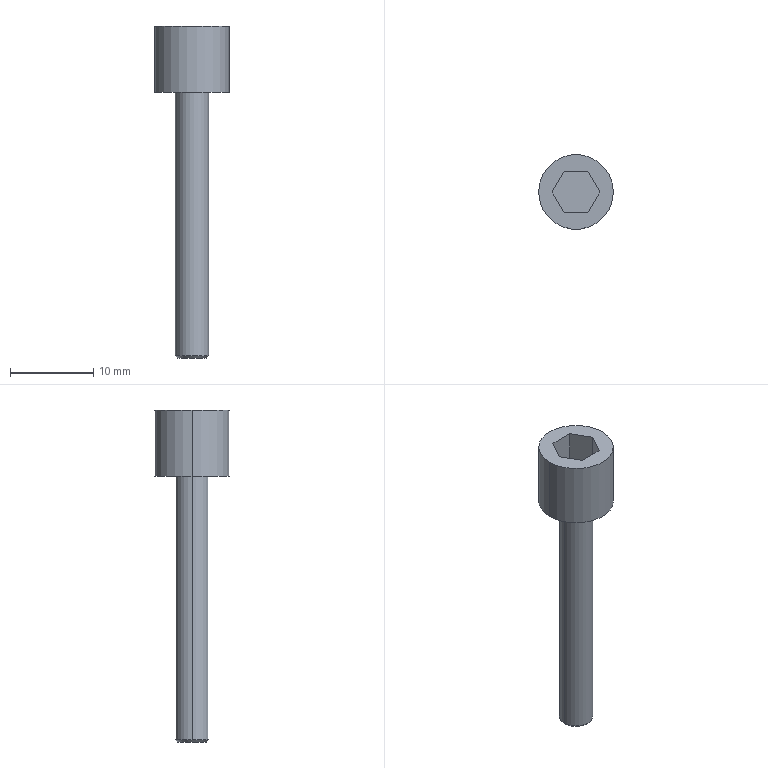Part | SolidWorks | features BaseBody 1 | 1 solid | 16 faces | box 9 x 9 x 40 mm | volume 802.432 mm3 | plane 10 | cylinder 4 | cone 2 | commonest cylinder face diameters 4 x2 9 x2
STEP:
#1=CARTESIAN_POINT('',(1.75,0.,-32.));
#2=VERTEX_POINT('',#1);
#3=CARTESIAN_POINT('',(-1.75,0.,-32.));
#4=VERTEX_POINT('',#3);
#5=CARTESIAN_POINT('',(0.,0.,-32.));
#6=DIRECTION('',(0.,0.,1.));
#7=DIRECTION('',(1.,0.,0.));
#8=AXIS2_PLACEMENT_3D('',#5,#6,#7);
#9=CIRCLE('',#8,1.75);
#10=EDGE_CURVE('',#2,#4,#9,.T.);
#11=ORIENTED_EDGE('',*,*,#10,.T.);
#12=CARTESIAN_POINT('',(-2.,0.,-31.75));
#13=VERTEX_POINT('',#12);
#14=CARTESIAN_POINT('',(-1.875,0.,-31.875));
#15=DIRECTION('',(-0.7071,0.,0.7071));
#16=VECTOR('',#15,1000.);
#17=LINE('',#14,#16);
#18=EDGE_CURVE('',#4,#13,#17,.T.);
#19=ORIENTED_EDGE('',*,*,#18,.T.);
#20=CARTESIAN_POINT('',(2.,0.,-31.75));
#21=VERTEX_POINT('',#20);
#22=CARTESIAN_POINT('',(0.,0.,-31.75));
#23=DIRECTION('',(0.,0.,-1.));
#24=DIRECTION('',(1.,0.,0.));
#25=AXIS2_PLACEMENT_3D('',#22,#23,#24);
#26=CIRCLE('',#25,2.);
#27=EDGE_CURVE('',#13,#21,#26,.T.);
#28=ORIENTED_EDGE('',*,*,#27,.T.);
#29=CARTESIAN_POINT('',(1.875,0.,-31.875));
#30=DIRECTION('',(0.7071,0.,0.7071));
#31=VECTOR('',#30,1000.);
#32=LINE('',#29,#31);
#33=EDGE_CURVE('',#2,#21,#32,.T.);
#34=ORIENTED_EDGE('',*,*,#33,.F.);
#35=EDGE_LOOP('',(#11,#19,#28,#34));
#36=FACE_OUTER_BOUND('',#35,.T.);
#37=CARTESIAN_POINT('',(0.,0.,-31.875));
#38=DIRECTION('',(0.,0.,1.));
#39=DIRECTION('',(1.,0.,0.));
#40=AXIS2_PLACEMENT_3D('',#37,#38,#39);
#41=CONICAL_SURFACE('',#40,1.875,0.7854);
#42=ADVANCED_FACE('',(#36),#41,.T.);
#43=ORIENTED_EDGE('',*,*,#27,.F.);
#44=CARTESIAN_POINT('',(-2.,0.,0.));
#45=VERTEX_POINT('',#44);
#46=CARTESIAN_POINT('',(-2.,0.,0.));
#47=DIRECTION('',(0.,0.,1.));
#48=VECTOR('',#47,1000.);
#49=LINE('',#46,#48);
#50=EDGE_CURVE('',#13,#45,#49,.T.);
#51=ORIENTED_EDGE('',*,*,#50,.T.);
#52=CARTESIAN_POINT('',(2.,0.,0.));
#53=VERTEX_POINT('',#52);
#54=CARTESIAN_POINT('',(0.,0.,0.));
#55=DIRECTION('',(0.,0.,1.));
#56=DIRECTION('',(1.,0.,0.));
#57=AXIS2_PLACEMENT_3D('',#54,#55,#56);
#58=CIRCLE('',#57,2.);
#59=EDGE_CURVE('',#53,#45,#58,.T.);
#60=ORIENTED_EDGE('',*,*,#59,.F.);
#61=CARTESIAN_POINT('',(2.,0.,0.));
#62=DIRECTION('',(0.,0.,1.));
#63=VECTOR('',#62,1000.);
#64=LINE('',#61,#63);
#65=EDGE_CURVE('',#21,#53,#64,.T.);
#66=ORIENTED_EDGE('',*,*,#65,.F.);
#67=EDGE_LOOP('',(#43,#51,#60,#66));
#68=FACE_OUTER_BOUND('',#67,.T.);
#69=CARTESIAN_POINT('',(0.,0.,0.));
#70=DIRECTION('',(0.,0.,1.));
#71=DIRECTION('',(1.,0.,0.));
#72=AXIS2_PLACEMENT_3D('',#69,#70,#71);
#73=CYLINDRICAL_SURFACE('',#72,2.);
#74=ADVANCED_FACE('',(#68),#73,.T.);
#75=CARTESIAN_POINT('',(4.5,0.,8.));
#76=VERTEX_POINT('',#75);
#77=CARTESIAN_POINT('',(-4.5,0.,8.));
#78=VERTEX_POINT('',#77);
#79=CARTESIAN_POINT('',(0.,0.,8.));
#80=DIRECTION('',(0.,0.,1.));
#81=DIRECTION('',(-1.,0.,0.));
#82=AXIS2_PLACEMENT_3D('',#79,#80,#81);
#83=CIRCLE('',#82,4.5);
#84=EDGE_CURVE('',#76,#78,#83,.T.);
#85=ORIENTED_EDGE('',*,*,#84,.F.);
#86=CARTESIAN_POINT('',(4.5,0.,0.));
#87=VERTEX_POINT('',#86);
#88=CARTESIAN_POINT('',(4.5,0.,0.));
#89=DIRECTION('',(0.,0.,-1.));
#90=VECTOR('',#89,1000.);
#91=LINE('',#88,#90);
#92=EDGE_CURVE('',#76,#87,#91,.T.);
#93=ORIENTED_EDGE('',*,*,#92,.T.);
#94=CARTESIAN_POINT('',(-4.5,0.,0.));
#95=VERTEX_POINT('',#94);
#96=CARTESIAN_POINT('',(0.,0.,0.));
#97=DIRECTION('',(0.,0.,-1.));
#98=DIRECTION('',(-1.,0.,0.));
#99=AXIS2_PLACEMENT_3D('',#96,#97,#98);
#100=CIRCLE('',#99,4.5);
#101=EDGE_CURVE('',#95,#87,#100,.T.);
#102=ORIENTED_EDGE('',*,*,#101,.F.);
#103=CARTESIAN_POINT('',(-4.5,0.,0.));
#104=DIRECTION('',(0.,0.,-1.));
#105=VECTOR('',#104,1000.);
#106=LINE('',#103,#105);
#107=EDGE_CURVE('',#78,#95,#106,.T.);
#108=ORIENTED_EDGE('',*,*,#107,.F.);
#109=EDGE_LOOP('',(#85,#93,#102,#108));
#110=FACE_OUTER_BOUND('',#109,.T.);
#111=CARTESIAN_POINT('',(0.,0.,0.));
#112=DIRECTION('',(0.,0.,-1.));
#113=DIRECTION('',(-1.,0.,0.));
#114=AXIS2_PLACEMENT_3D('',#111,#112,#113);
#115=CYLINDRICAL_SURFACE('',#114,4.5);
#116=ADVANCED_FACE('',(#110),#115,.T.);
#117=CARTESIAN_POINT('',(2.887,0.,8.));
#118=VERTEX_POINT('',#117);
#119=CARTESIAN_POINT('',(1.443,-2.5,8.));
#120=VERTEX_POINT('',#119);
#121=CARTESIAN_POINT('',(2.526,-0.625,8.));
#122=DIRECTION('',(-0.5,-0.866,0.));
#123=VECTOR('',#122,1000.);
#124=LINE('',#121,#123);
#125=EDGE_CURVE('',#118,#120,#124,.T.);
#126=ORIENTED_EDGE('',*,*,#125,.F.);
#127=CARTESIAN_POINT('',(2.887,0.,3.));
#128=VERTEX_POINT('',#127);
#129=CARTESIAN_POINT('',(2.887,0.,8.));
#130=DIRECTION('',(0.,0.,-1.));
#131=VECTOR('',#130,1000.);
#132=LINE('',#129,#131);
#133=EDGE_CURVE('',#118,#128,#132,.T.);
#134=ORIENTED_EDGE('',*,*,#133,.T.);
#135=CARTESIAN_POINT('',(1.443,-2.5,3.));
#136=VERTEX_POINT('',#135);
#137=CARTESIAN_POINT('',(2.887,0.,3.));
#138=DIRECTION('',(-0.5,-0.866,0.));
#139=VECTOR('',#138,1000.);
#140=LINE('',#137,#139);
#141=EDGE_CURVE('',#128,#136,#140,.T.);
#142=ORIENTED_EDGE('',*,*,#141,.T.);
#143=CARTESIAN_POINT('',(1.443,-2.5,8.));
#144=DIRECTION('',(0.,0.,-1.));
#145=VECTOR('',#144,1000.);
#146=LINE('',#143,#145);
#147=EDGE_CURVE('',#120,#136,#146,.T.);
#148=ORIENTED_EDGE('',*,*,#147,.F.);
#149=EDGE_LOOP('',(#126,#134,#142,#148));
#150=FACE_OUTER_BOUND('',#149,.T.);
#151=CARTESIAN_POINT('',(2.887,0.,8.));
#152=DIRECTION('',(0.866,-0.5,0.));
#153=DIRECTION('',(0.,0.,-1.));
#154=AXIS2_PLACEMENT_3D('',#151,#152,#153);
#155=PLANE('',#154);
#156=ADVANCED_FACE('',(#150),#155,.F.);
#157=CARTESIAN_POINT('',(1.443,2.5,8.));
#158=VERTEX_POINT('',#157);
#159=CARTESIAN_POINT('',(1.804,1.875,8.));
#160=DIRECTION('',(0.5,-0.866,0.));
#161=VECTOR('',#160,1000.);
#162=LINE('',#159,#161);
#163=EDGE_CURVE('',#158,#118,#162,.T.);
#164=ORIENTED_EDGE('',*,*,#163,.F.);
#165=CARTESIAN_POINT('',(1.443,2.5,3.));
#166=VERTEX_POINT('',#165);
#167=CARTESIAN_POINT('',(1.443,2.5,8.));
#168=DIRECTION('',(0.,0.,-1.));
#169=VECTOR('',#168,1000.);
#170=LINE('',#167,#169);
#171=EDGE_CURVE('',#158,#166,#170,.T.);
#172=ORIENTED_EDGE('',*,*,#171,.T.);
#173=CARTESIAN_POINT('',(1.443,2.5,3.));
#174=DIRECTION('',(0.5,-0.866,0.));
#175=VECTOR('',#174,1000.);
#176=LINE('',#173,#175);
#177=EDGE_CURVE('',#166,#128,#176,.T.);
#178=ORIENTED_EDGE('',*,*,#177,.T.);
#179=ORIENTED_EDGE('',*,*,#133,.F.);
#180=EDGE_LOOP('',(#164,#172,#178,#179));
#181=FACE_OUTER_BOUND('',#180,.T.);
#182=CARTESIAN_POINT('',(1.443,2.5,8.));
#183=DIRECTION('',(0.866,0.5,0.));
#184=DIRECTION('',(0.,0.,-1.));
#185=AXIS2_PLACEMENT_3D('',#182,#183,#184);
#186=PLANE('',#185);
#187=ADVANCED_FACE('',(#181),#186,.F.);
#188=CARTESIAN_POINT('',(-1.443,2.5,8.));
#189=VERTEX_POINT('',#188);
#190=CARTESIAN_POINT('',(-0.7217,2.5,8.));
#191=DIRECTION('',(1.,0.,0.));
#192=VECTOR('',#191,1000.);
#193=LINE('',#190,#192);
#194=EDGE_CURVE('',#189,#158,#193,.T.);
#195=ORIENTED_EDGE('',*,*,#194,.F.);
#196=CARTESIAN_POINT('',(-1.443,2.5,3.));
#197=VERTEX_POINT('',#196);
#198=CARTESIAN_POINT('',(-1.443,2.5,8.));
#199=DIRECTION('',(0.,0.,-1.));
#200=VECTOR('',#199,1000.);
#201=LINE('',#198,#200);
#202=EDGE_CURVE('',#189,#197,#201,.T.);
#203=ORIENTED_EDGE('',*,*,#202,.T.);
#204=CARTESIAN_POINT('',(-1.443,2.5,3.));
#205=DIRECTION('',(1.,0.,0.));
#206=VECTOR('',#205,1000.);
#207=LINE('',#204,#206);
#208=EDGE_CURVE('',#197,#166,#207,.T.);
#209=ORIENTED_EDGE('',*,*,#208,.T.);
#210=ORIENTED_EDGE('',*,*,#171,.F.);
#211=EDGE_LOOP('',(#195,#203,#209,#210));
#212=FACE_OUTER_BOUND('',#211,.T.);
#213=CARTESIAN_POINT('',(-1.443,2.5,8.));
#214=DIRECTION('',(0.,1.,0.));
#215=DIRECTION('',(1.,0.,0.));
#216=AXIS2_PLACEMENT_3D('',#213,#214,#215);
#217=PLANE('',#216);
#218=ADVANCED_FACE('',(#212),#217,.F.);
#219=CARTESIAN_POINT('',(-2.887,0.,8.));
#220=VERTEX_POINT('',#219);
#221=CARTESIAN_POINT('',(-2.526,0.625,8.));
#222=DIRECTION('',(0.5,0.866,0.));
#223=VECTOR('',#222,1000.);
#224=LINE('',#221,#223);
#225=EDGE_CURVE('',#220,#189,#224,.T.);
#226=ORIENTED_EDGE('',*,*,#225,.F.);
#227=CARTESIAN_POINT('',(-2.887,0.,3.));
#228=VERTEX_POINT('',#227);
#229=CARTESIAN_POINT('',(-2.887,0.,8.));
#230=DIRECTION('',(0.,0.,-1.));
#231=VECTOR('',#230,1000.);
#232=LINE('',#229,#231);
#233=EDGE_CURVE('',#220,#228,#232,.T.);
#234=ORIENTED_EDGE('',*,*,#233,.T.);
#235=CARTESIAN_POINT('',(-2.887,0.,3.));
#236=DIRECTION('',(0.5,0.866,0.));
#237=VECTOR('',#236,1000.);
#238=LINE('',#235,#237);
#239=EDGE_CURVE('',#228,#197,#238,.T.);
#240=ORIENTED_EDGE('',*,*,#239,.T.);
#241=ORIENTED_EDGE('',*,*,#202,.F.);
#242=EDGE_LOOP('',(#226,#234,#240,#241));
#243=FACE_OUTER_BOUND('',#242,.T.);
#244=CARTESIAN_POINT('',(-2.887,0.,8.));
#245=DIRECTION('',(-0.866,0.5,0.));
#246=DIRECTION('',(0.,0.,1.));
#247=AXIS2_PLACEMENT_3D('',#244,#245,#246);
#248=PLANE('',#247);
#249=ADVANCED_FACE('',(#243),#248,.F.);
#250=CARTESIAN_POINT('',(-1.443,-2.5,8.));
#251=VERTEX_POINT('',#250);
#252=CARTESIAN_POINT('',(-1.804,-1.875,8.));
#253=DIRECTION('',(-0.5,0.866,0.));
#254=VECTOR('',#253,1000.);
#255=LINE('',#252,#254);
#256=EDGE_CURVE('',#251,#220,#255,.T.);
#257=ORIENTED_EDGE('',*,*,#256,.F.);
#258=CARTESIAN_POINT('',(-1.443,-2.5,3.));
#259=VERTEX_POINT('',#258);
#260=CARTESIAN_POINT('',(-1.443,-2.5,8.));
#261=DIRECTION('',(0.,0.,-1.));
#262=VECTOR('',#261,1000.);
#263=LINE('',#260,#262);
#264=EDGE_CURVE('',#251,#259,#263,.T.);
#265=ORIENTED_EDGE('',*,*,#264,.T.);
#266=CARTESIAN_POINT('',(-1.443,-2.5,3.));
#267=DIRECTION('',(-0.5,0.866,0.));
#268=VECTOR('',#267,1000.);
#269=LINE('',#266,#268);
#270=EDGE_CURVE('',#259,#228,#269,.T.);
#271=ORIENTED_EDGE('',*,*,#270,.T.);
#272=ORIENTED_EDGE('',*,*,#233,.F.);
#273=EDGE_LOOP('',(#257,#265,#271,#272));
#274=FACE_OUTER_BOUND('',#273,.T.);
#275=CARTESIAN_POINT('',(-1.443,-2.5,8.));
#276=DIRECTION('',(-0.866,-0.5,0.));
#277=DIRECTION('',(-0.5,0.866,0.));
#278=AXIS2_PLACEMENT_3D('',#275,#276,#277);
#279=PLANE('',#278);
#280=ADVANCED_FACE('',(#274),#279,.F.);
#281=CARTESIAN_POINT('',(0.7217,-2.5,8.));
#282=DIRECTION('',(-1.,0.,0.));
#283=VECTOR('',#282,1000.);
#284=LINE('',#281,#283);
#285=EDGE_CURVE('',#120,#251,#284,.T.);
#286=ORIENTED_EDGE('',*,*,#285,.F.);
#287=ORIENTED_EDGE('',*,*,#147,.T.);
#288=CARTESIAN_POINT('',(1.443,-2.5,3.));
#289=DIRECTION('',(-1.,0.,0.));
#290=VECTOR('',#289,1000.);
#291=LINE('',#288,#290);
#292=EDGE_CURVE('',#136,#259,#291,.T.);
#293=ORIENTED_EDGE('',*,*,#292,.T.);
#294=ORIENTED_EDGE('',*,*,#264,.F.);
#295=EDGE_LOOP('',(#286,#287,#293,#294));
#296=FACE_OUTER_BOUND('',#295,.T.);
#297=CARTESIAN_POINT('',(1.443,-2.5,8.));
#298=DIRECTION('',(0.,-1.,0.));
#299=DIRECTION('',(-1.,0.,0.));
#300=AXIS2_PLACEMENT_3D('',#297,#298,#299);
#301=PLANE('',#300);
#302=ADVANCED_FACE('',(#296),#301,.F.);
#303=ORIENTED_EDGE('',*,*,#292,.F.);
#304=ORIENTED_EDGE('',*,*,#141,.F.);
#305=ORIENTED_EDGE('',*,*,#177,.F.);
#306=ORIENTED_EDGE('',*,*,#208,.F.);
#307=ORIENTED_EDGE('',*,*,#239,.F.);
#308=ORIENTED_EDGE('',*,*,#270,.F.);
#309=EDGE_LOOP('',(#303,#304,#305,#306,#307,#308));
#310=FACE_OUTER_BOUND('',#309,.T.);
#311=CARTESIAN_POINT('',(0.,0.,3.));
#312=DIRECTION('',(0.,0.,-1.));
#313=DIRECTION('',(0.,-1.,0.));
#314=AXIS2_PLACEMENT_3D('',#311,#312,#313);
#315=PLANE('',#314);
#316=ADVANCED_FACE('',(#310),#315,.F.);
#317=ORIENTED_EDGE('',*,*,#10,.F.);
#318=CARTESIAN_POINT('',(0.,0.,-32.));
#319=DIRECTION('',(0.,0.,1.));
#320=DIRECTION('',(1.,0.,0.));
#321=AXIS2_PLACEMENT_3D('',#318,#319,#320);
#322=CIRCLE('',#321,1.75);
#323=EDGE_CURVE('',#4,#2,#322,.T.);
#324=ORIENTED_EDGE('',*,*,#323,.F.);
#325=EDGE_LOOP('',(#317,#324));
#326=FACE_OUTER_BOUND('',#325,.T.);
#327=CARTESIAN_POINT('',(0.,0.,-32.));
#328=DIRECTION('',(0.,0.,1.));
#329=DIRECTION('',(1.,0.,0.));
#330=AXIS2_PLACEMENT_3D('',#327,#328,#329);
#331=PLANE('',#330);
#332=ADVANCED_FACE('',(#326),#331,.F.);
#333=ORIENTED_EDGE('',*,*,#59,.T.);
#334=CARTESIAN_POINT('',(0.,0.,0.));
#335=DIRECTION('',(0.,0.,1.));
#336=DIRECTION('',(1.,0.,0.));
#337=AXIS2_PLACEMENT_3D('',#334,#335,#336);
#338=CIRCLE('',#337,2.);
#339=EDGE_CURVE('',#45,#53,#338,.T.);
#340=ORIENTED_EDGE('',*,*,#339,.T.);
#341=EDGE_LOOP('',(#333,#340));
#342=FACE_BOUND('',#341,.T.);
#343=ORIENTED_EDGE('',*,*,#101,.T.);
#344=CARTESIAN_POINT('',(0.,0.,0.));
#345=DIRECTION('',(0.,0.,-1.));
#346=DIRECTION('',(-1.,0.,0.));
#347=AXIS2_PLACEMENT_3D('',#344,#345,#346);
#348=CIRCLE('',#347,4.5);
#349=EDGE_CURVE('',#87,#95,#348,.T.);
#350=ORIENTED_EDGE('',*,*,#349,.T.);
#351=EDGE_LOOP('',(#343,#350));
#352=FACE_OUTER_BOUND('',#351,.T.);
#353=CARTESIAN_POINT('',(0.,0.,0.));
#354=DIRECTION('',(0.,0.,1.));
#355=DIRECTION('',(1.,0.,0.));
#356=AXIS2_PLACEMENT_3D('',#353,#354,#355);
#357=PLANE('',#356);
#358=ADVANCED_FACE('',(#342,#352),#357,.F.);
#359=ORIENTED_EDGE('',*,*,#125,.T.);
#360=ORIENTED_EDGE('',*,*,#285,.T.);
#361=ORIENTED_EDGE('',*,*,#256,.T.);
#362=ORIENTED_EDGE('',*,*,#225,.T.);
#363=ORIENTED_EDGE('',*,*,#194,.T.);
#364=ORIENTED_EDGE('',*,*,#163,.T.);
#365=EDGE_LOOP('',(#359,#360,#361,#362,#363,#364));
#366=FACE_BOUND('',#365,.T.);
#367=CARTESIAN_POINT('',(0.,0.,8.));
#368=DIRECTION('',(0.,0.,1.));
#369=DIRECTION('',(-1.,0.,0.));
#370=AXIS2_PLACEMENT_3D('',#367,#368,#369);
#371=CIRCLE('',#370,4.5);
#372=EDGE_CURVE('',#78,#76,#371,.T.);
#373=ORIENTED_EDGE('',*,*,#372,.T.);
#374=ORIENTED_EDGE('',*,*,#84,.T.);
#375=EDGE_LOOP('',(#373,#374));
#376=FACE_OUTER_BOUND('',#375,.T.);
#377=CARTESIAN_POINT('',(0.,0.,8.));
#378=DIRECTION('',(0.,0.,1.));
#379=DIRECTION('',(1.,0.,0.));
#380=AXIS2_PLACEMENT_3D('',#377,#378,#379);
#381=PLANE('',#380);
#382=ADVANCED_FACE('',(#366,#376),#381,.T.);
#383=ORIENTED_EDGE('',*,*,#92,.F.);
#384=ORIENTED_EDGE('',*,*,#372,.F.);
#385=ORIENTED_EDGE('',*,*,#107,.T.);
#386=ORIENTED_EDGE('',*,*,#349,.F.);
#387=EDGE_LOOP('',(#383,#384,#385,#386));
#388=FACE_OUTER_BOUND('',#387,.T.);
#389=CARTESIAN_POINT('',(0.,0.,0.));
#390=DIRECTION('',(0.,0.,-1.));
#391=DIRECTION('',(-1.,0.,0.));
#392=AXIS2_PLACEMENT_3D('',#389,#390,#391);
#393=CYLINDRICAL_SURFACE('',#392,4.5);
#394=ADVANCED_FACE('',(#388),#393,.T.);
#395=ORIENTED_EDGE('',*,*,#50,.F.);
#396=CARTESIAN_POINT('',(0.,0.,-31.75));
#397=DIRECTION('',(0.,0.,-1.));
#398=DIRECTION('',(1.,0.,0.));
#399=AXIS2_PLACEMENT_3D('',#396,#397,#398);
#400=CIRCLE('',#399,2.);
#401=EDGE_CURVE('',#21,#13,#400,.T.);
#402=ORIENTED_EDGE('',*,*,#401,.F.);
#403=ORIENTED_EDGE('',*,*,#65,.T.);
#404=ORIENTED_EDGE('',*,*,#339,.F.);
#405=EDGE_LOOP('',(#395,#402,#403,#404));
#406=FACE_OUTER_BOUND('',#405,.T.);
#407=CARTESIAN_POINT('',(0.,0.,0.));
#408=DIRECTION('',(0.,0.,1.));
#409=DIRECTION('',(1.,0.,0.));
#410=AXIS2_PLACEMENT_3D('',#407,#408,#409);
#411=CYLINDRICAL_SURFACE('',#410,2.);
#412=ADVANCED_FACE('',(#406),#411,.T.);
#413=ORIENTED_EDGE('',*,*,#18,.F.);
#414=ORIENTED_EDGE('',*,*,#323,.T.);
#415=ORIENTED_EDGE('',*,*,#33,.T.);
#416=ORIENTED_EDGE('',*,*,#401,.T.);
#417=EDGE_LOOP('',(#413,#414,#415,#416));
#418=FACE_OUTER_BOUND('',#417,.T.);
#419=CARTESIAN_POINT('',(0.,0.,-31.875));
#420=DIRECTION('',(0.,0.,1.));
#421=DIRECTION('',(1.,0.,0.));
#422=AXIS2_PLACEMENT_3D('',#419,#420,#421);
#423=CONICAL_SURFACE('',#422,1.875,0.7854);
#424=ADVANCED_FACE('',(#418),#423,.T.);
#425=CLOSED_SHELL('',(#42,#74,#116,#156,#187,#218,#249,#280,#302,#316,#332,#358,#382,#394,#412,#424));
#426=MANIFOLD_SOLID_BREP('',#425);
#427=CARTESIAN_POINT('',(0.,0.,0.));
#428=DIRECTION('',(0.,0.,1.));
#429=DIRECTION('',(1.,0.,0.));
#430=AXIS2_PLACEMENT_3D('',#427,#428,#429);
#431=(LENGTH_UNIT()NAMED_UNIT(*)SI_UNIT(.MILLI.,.METRE.));
#432=UNCERTAINTY_MEASURE_WITH_UNIT(LENGTH_MEASURE(0.00001),#431,'','');
#433=(NAMED_UNIT(*)PLANE_ANGLE_UNIT()SI_UNIT($,.RADIAN.));
#434=(NAMED_UNIT(*)SI_UNIT($,.STERADIAN.)SOLID_ANGLE_UNIT());
#435=(GEOMETRIC_REPRESENTATION_CONTEXT(3)GLOBAL_UNCERTAINTY_ASSIGNED_CONTEXT((#432))GLOBAL_UNIT_ASSIGNED_CONTEXT((#431,#433,#434))REPRESENTATION_CONTEXT('',''));
#436=ADVANCED_BREP_SHAPE_REPRESENTATION('',(#426,#430),#435);